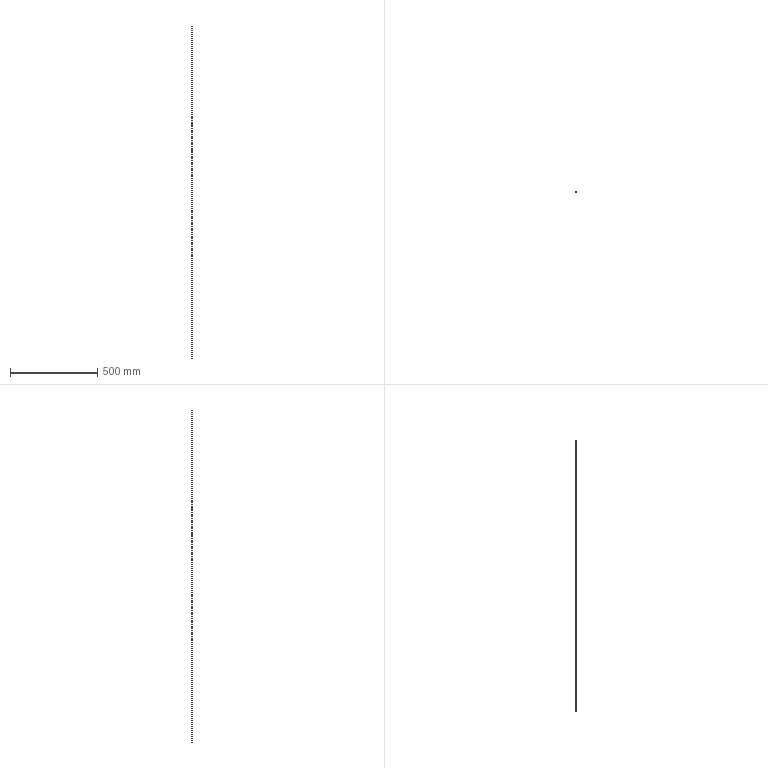Part | SolidWorks | features Extrusion 1 | 1 solid | 6 faces | box 0.3 x 0.3 x 1900 mm | volume 100.727 mm3 | cylinder 4 | plane 2 | commonest cylinder face diameters 0.15 x2 0.3 x2
STEP:
#1=CARTESIAN_POINT('',(-0.075,0.,1900.));
#2=VERTEX_POINT('',#1);
#3=CARTESIAN_POINT('',(0.075,0.,1900.));
#4=VERTEX_POINT('',#3);
#5=CARTESIAN_POINT('',(0.,0.,1900.));
#6=DIRECTION('',(0.,0.,1.));
#7=DIRECTION('',(1.,0.,0.));
#8=AXIS2_PLACEMENT_3D('',#5,#6,#7);
#9=CIRCLE('',#8,0.075);
#10=EDGE_CURVE('',#2,#4,#9,.T.);
#11=ORIENTED_EDGE('',*,*,#10,.T.);
#12=CARTESIAN_POINT('',(0.075,0.,0.));
#13=VERTEX_POINT('',#12);
#14=CARTESIAN_POINT('',(0.075,0.,1900.));
#15=DIRECTION('',(0.,0.,-1.));
#16=VECTOR('',#15,1000.);
#17=LINE('',#14,#16);
#18=EDGE_CURVE('',#4,#13,#17,.T.);
#19=ORIENTED_EDGE('',*,*,#18,.T.);
#20=CARTESIAN_POINT('',(-0.075,0.,0.));
#21=VERTEX_POINT('',#20);
#22=CARTESIAN_POINT('',(0.,0.,0.));
#23=DIRECTION('',(0.,0.,1.));
#24=DIRECTION('',(1.,0.,0.));
#25=AXIS2_PLACEMENT_3D('',#22,#23,#24);
#26=CIRCLE('',#25,0.075);
#27=EDGE_CURVE('',#21,#13,#26,.T.);
#28=ORIENTED_EDGE('',*,*,#27,.F.);
#29=CARTESIAN_POINT('',(-0.075,0.,1900.));
#30=DIRECTION('',(0.,0.,-1.));
#31=VECTOR('',#30,1000.);
#32=LINE('',#29,#31);
#33=EDGE_CURVE('',#2,#21,#32,.T.);
#34=ORIENTED_EDGE('',*,*,#33,.F.);
#35=EDGE_LOOP('',(#11,#19,#28,#34));
#36=FACE_OUTER_BOUND('',#35,.T.);
#37=CARTESIAN_POINT('',(0.,0.,1900.));
#38=DIRECTION('',(0.,0.,-1.));
#39=DIRECTION('',(-1.,0.,0.));
#40=AXIS2_PLACEMENT_3D('',#37,#38,#39);
#41=CYLINDRICAL_SURFACE('',#40,0.075);
#42=ADVANCED_FACE('',(#36),#41,.F.);
#43=CARTESIAN_POINT('',(0.15,0.,1900.));
#44=VERTEX_POINT('',#43);
#45=CARTESIAN_POINT('',(-0.15,0.,1900.));
#46=VERTEX_POINT('',#45);
#47=CARTESIAN_POINT('',(0.,0.,1900.));
#48=DIRECTION('',(0.,0.,1.));
#49=DIRECTION('',(1.,0.,0.));
#50=AXIS2_PLACEMENT_3D('',#47,#48,#49);
#51=CIRCLE('',#50,0.15);
#52=EDGE_CURVE('',#44,#46,#51,.T.);
#53=ORIENTED_EDGE('',*,*,#52,.F.);
#54=CARTESIAN_POINT('',(0.15,0.,0.));
#55=VERTEX_POINT('',#54);
#56=CARTESIAN_POINT('',(0.15,0.,1900.));
#57=DIRECTION('',(0.,0.,-1.));
#58=VECTOR('',#57,1000.);
#59=LINE('',#56,#58);
#60=EDGE_CURVE('',#44,#55,#59,.T.);
#61=ORIENTED_EDGE('',*,*,#60,.T.);
#62=CARTESIAN_POINT('',(-0.15,0.,0.));
#63=VERTEX_POINT('',#62);
#64=CARTESIAN_POINT('',(0.,0.,0.));
#65=DIRECTION('',(0.,0.,1.));
#66=DIRECTION('',(1.,0.,0.));
#67=AXIS2_PLACEMENT_3D('',#64,#65,#66);
#68=CIRCLE('',#67,0.15);
#69=EDGE_CURVE('',#55,#63,#68,.T.);
#70=ORIENTED_EDGE('',*,*,#69,.T.);
#71=CARTESIAN_POINT('',(-0.15,0.,1900.));
#72=DIRECTION('',(0.,0.,-1.));
#73=VECTOR('',#72,1000.);
#74=LINE('',#71,#73);
#75=EDGE_CURVE('',#46,#63,#74,.T.);
#76=ORIENTED_EDGE('',*,*,#75,.F.);
#77=EDGE_LOOP('',(#53,#61,#70,#76));
#78=FACE_OUTER_BOUND('',#77,.T.);
#79=CARTESIAN_POINT('',(0.,0.,1900.));
#80=DIRECTION('',(0.,0.,-1.));
#81=DIRECTION('',(-1.,0.,0.));
#82=AXIS2_PLACEMENT_3D('',#79,#80,#81);
#83=CYLINDRICAL_SURFACE('',#82,0.15);
#84=ADVANCED_FACE('',(#78),#83,.T.);
#85=CARTESIAN_POINT('',(0.,0.,1900.));
#86=DIRECTION('',(0.,0.,1.));
#87=DIRECTION('',(1.,0.,0.));
#88=AXIS2_PLACEMENT_3D('',#85,#86,#87);
#89=CIRCLE('',#88,0.15);
#90=EDGE_CURVE('',#46,#44,#89,.T.);
#91=ORIENTED_EDGE('',*,*,#90,.T.);
#92=ORIENTED_EDGE('',*,*,#52,.T.);
#93=EDGE_LOOP('',(#91,#92));
#94=FACE_OUTER_BOUND('',#93,.T.);
#95=ORIENTED_EDGE('',*,*,#10,.F.);
#96=CARTESIAN_POINT('',(0.,0.,1900.));
#97=DIRECTION('',(0.,0.,1.));
#98=DIRECTION('',(1.,0.,0.));
#99=AXIS2_PLACEMENT_3D('',#96,#97,#98);
#100=CIRCLE('',#99,0.075);
#101=EDGE_CURVE('',#4,#2,#100,.T.);
#102=ORIENTED_EDGE('',*,*,#101,.F.);
#103=EDGE_LOOP('',(#95,#102));
#104=FACE_BOUND('',#103,.T.);
#105=CARTESIAN_POINT('',(0.,0.,1900.));
#106=DIRECTION('',(0.,0.,1.));
#107=DIRECTION('',(1.,0.,0.));
#108=AXIS2_PLACEMENT_3D('',#105,#106,#107);
#109=PLANE('',#108);
#110=ADVANCED_FACE('',(#94,#104),#109,.T.);
#111=CARTESIAN_POINT('',(0.,0.,0.));
#112=DIRECTION('',(0.,0.,1.));
#113=DIRECTION('',(1.,0.,0.));
#114=AXIS2_PLACEMENT_3D('',#111,#112,#113);
#115=CIRCLE('',#114,0.15);
#116=EDGE_CURVE('',#63,#55,#115,.T.);
#117=ORIENTED_EDGE('',*,*,#116,.F.);
#118=ORIENTED_EDGE('',*,*,#69,.F.);
#119=EDGE_LOOP('',(#117,#118));
#120=FACE_OUTER_BOUND('',#119,.T.);
#121=ORIENTED_EDGE('',*,*,#27,.T.);
#122=CARTESIAN_POINT('',(0.,0.,0.));
#123=DIRECTION('',(0.,0.,1.));
#124=DIRECTION('',(1.,0.,0.));
#125=AXIS2_PLACEMENT_3D('',#122,#123,#124);
#126=CIRCLE('',#125,0.075);
#127=EDGE_CURVE('',#13,#21,#126,.T.);
#128=ORIENTED_EDGE('',*,*,#127,.T.);
#129=EDGE_LOOP('',(#121,#128));
#130=FACE_BOUND('',#129,.T.);
#131=CARTESIAN_POINT('',(0.,0.,0.));
#132=DIRECTION('',(0.,0.,1.));
#133=DIRECTION('',(1.,0.,0.));
#134=AXIS2_PLACEMENT_3D('',#131,#132,#133);
#135=PLANE('',#134);
#136=ADVANCED_FACE('',(#120,#130),#135,.F.);
#137=ORIENTED_EDGE('',*,*,#60,.F.);
#138=ORIENTED_EDGE('',*,*,#90,.F.);
#139=ORIENTED_EDGE('',*,*,#75,.T.);
#140=ORIENTED_EDGE('',*,*,#116,.T.);
#141=EDGE_LOOP('',(#137,#138,#139,#140));
#142=FACE_OUTER_BOUND('',#141,.T.);
#143=CARTESIAN_POINT('',(0.,0.,1900.));
#144=DIRECTION('',(0.,0.,-1.));
#145=DIRECTION('',(-1.,0.,0.));
#146=AXIS2_PLACEMENT_3D('',#143,#144,#145);
#147=CYLINDRICAL_SURFACE('',#146,0.15);
#148=ADVANCED_FACE('',(#142),#147,.T.);
#149=ORIENTED_EDGE('',*,*,#18,.F.);
#150=ORIENTED_EDGE('',*,*,#101,.T.);
#151=ORIENTED_EDGE('',*,*,#33,.T.);
#152=ORIENTED_EDGE('',*,*,#127,.F.);
#153=EDGE_LOOP('',(#149,#150,#151,#152));
#154=FACE_OUTER_BOUND('',#153,.T.);
#155=CARTESIAN_POINT('',(0.,0.,1900.));
#156=DIRECTION('',(0.,0.,-1.));
#157=DIRECTION('',(-1.,0.,0.));
#158=AXIS2_PLACEMENT_3D('',#155,#156,#157);
#159=CYLINDRICAL_SURFACE('',#158,0.075);
#160=ADVANCED_FACE('',(#154),#159,.F.);
#161=CLOSED_SHELL('',(#42,#84,#110,#136,#148,#160));
#162=MANIFOLD_SOLID_BREP('',#161);
#163=CARTESIAN_POINT('',(0.,0.,0.));
#164=DIRECTION('',(0.,0.,1.));
#165=DIRECTION('',(1.,0.,0.));
#166=AXIS2_PLACEMENT_3D('',#163,#164,#165);
#167=(LENGTH_UNIT()NAMED_UNIT(*)SI_UNIT(.MILLI.,.METRE.));
#168=UNCERTAINTY_MEASURE_WITH_UNIT(LENGTH_MEASURE(0.00001),#167,'','');
#169=(NAMED_UNIT(*)PLANE_ANGLE_UNIT()SI_UNIT($,.RADIAN.));
#170=(NAMED_UNIT(*)SI_UNIT($,.STERADIAN.)SOLID_ANGLE_UNIT());
#171=(GEOMETRIC_REPRESENTATION_CONTEXT(3)GLOBAL_UNCERTAINTY_ASSIGNED_CONTEXT((#168))GLOBAL_UNIT_ASSIGNED_CONTEXT((#167,#169,#170))REPRESENTATION_CONTEXT('',''));
#172=ADVANCED_BREP_SHAPE_REPRESENTATION('',(#162,#166),#171);